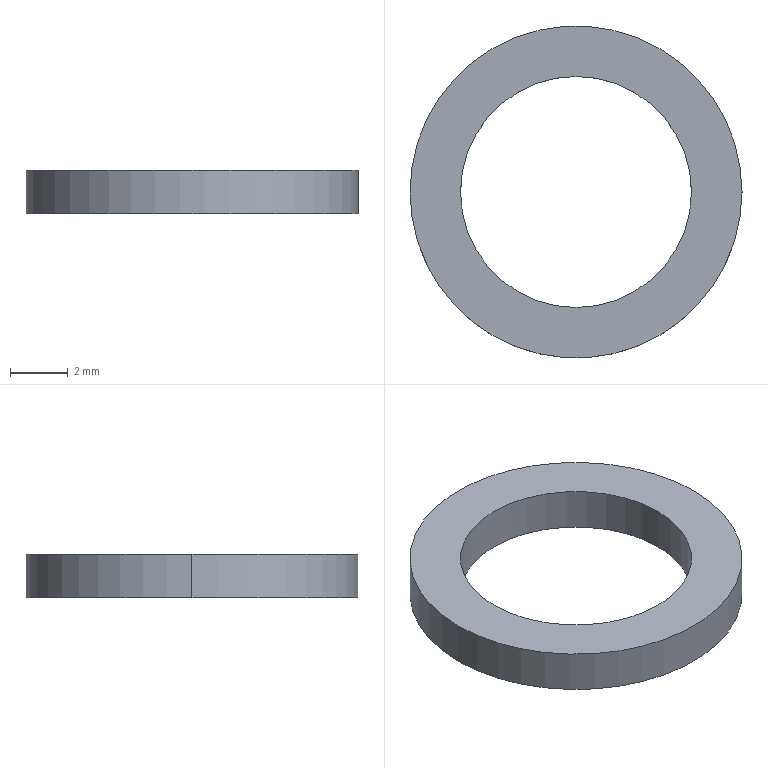Part | NX | features BREP 1 | 1 solid | 6 faces | box 11.5 x 11.5 x 1.5 mm | volume 80.405 mm3 | cylinder 4 | plane 2 | commonest cylinder face diameters 8 x2 11.5 x2
STEP:
#1=CARTESIAN_POINT('',(4.,0.,1.5));
#2=VERTEX_POINT('',#1);
#3=CARTESIAN_POINT('',(4.,0.,0.));
#4=VERTEX_POINT('',#3);
#5=CARTESIAN_POINT('',(4.,0.,1.5));
#6=DIRECTION('',(0.,0.,-1.));
#7=VECTOR('',#6,1000.);
#8=LINE('',#5,#7);
#9=EDGE_CURVE('',#2,#4,#8,.T.);
#10=ORIENTED_EDGE('',*,*,#9,.F.);
#11=CARTESIAN_POINT('',(-4.,0.,1.5));
#12=VERTEX_POINT('',#11);
#13=CARTESIAN_POINT('',(0.,0.,1.5));
#14=DIRECTION('',(0.,0.,1.));
#15=DIRECTION('',(1.,0.,0.));
#16=AXIS2_PLACEMENT_3D('',#13,#14,#15);
#17=CIRCLE('',#16,4.);
#18=EDGE_CURVE('',#2,#12,#17,.T.);
#19=ORIENTED_EDGE('',*,*,#18,.T.);
#20=CARTESIAN_POINT('',(-4.,0.,0.));
#21=VERTEX_POINT('',#20);
#22=CARTESIAN_POINT('',(-4.,0.,1.5));
#23=DIRECTION('',(0.,0.,-1.));
#24=VECTOR('',#23,1000.);
#25=LINE('',#22,#24);
#26=EDGE_CURVE('',#12,#21,#25,.T.);
#27=ORIENTED_EDGE('',*,*,#26,.T.);
#28=CARTESIAN_POINT('',(0.,0.,0.));
#29=DIRECTION('',(0.,0.,1.));
#30=DIRECTION('',(1.,0.,0.));
#31=AXIS2_PLACEMENT_3D('',#28,#29,#30);
#32=CIRCLE('',#31,4.);
#33=EDGE_CURVE('',#4,#21,#32,.T.);
#34=ORIENTED_EDGE('',*,*,#33,.F.);
#35=EDGE_LOOP('',(#10,#19,#27,#34));
#36=FACE_BOUND('',#35,.T.);
#37=CARTESIAN_POINT('',(0.,0.,1.5));
#38=DIRECTION('',(0.,0.,-1.));
#39=DIRECTION('',(-1.,0.,0.));
#40=AXIS2_PLACEMENT_3D('',#37,#38,#39);
#41=CYLINDRICAL_SURFACE('',#40,4.);
#42=ADVANCED_FACE('',(#36),#41,.F.);
#43=CARTESIAN_POINT('',(5.75,0.,1.5));
#44=VERTEX_POINT('',#43);
#45=CARTESIAN_POINT('',(5.75,0.,0.));
#46=VERTEX_POINT('',#45);
#47=CARTESIAN_POINT('',(5.75,0.,1.5));
#48=DIRECTION('',(0.,0.,-1.));
#49=VECTOR('',#48,1000.);
#50=LINE('',#47,#49);
#51=EDGE_CURVE('',#44,#46,#50,.T.);
#52=ORIENTED_EDGE('',*,*,#51,.F.);
#53=CARTESIAN_POINT('',(-5.75,0.,1.5));
#54=VERTEX_POINT('',#53);
#55=CARTESIAN_POINT('',(0.,0.,1.5));
#56=DIRECTION('',(0.,0.,1.));
#57=DIRECTION('',(1.,0.,0.));
#58=AXIS2_PLACEMENT_3D('',#55,#56,#57);
#59=CIRCLE('',#58,5.75);
#60=EDGE_CURVE('',#54,#44,#59,.T.);
#61=ORIENTED_EDGE('',*,*,#60,.F.);
#62=CARTESIAN_POINT('',(-5.75,0.,0.));
#63=VERTEX_POINT('',#62);
#64=CARTESIAN_POINT('',(-5.75,0.,1.5));
#65=DIRECTION('',(0.,0.,-1.));
#66=VECTOR('',#65,1000.);
#67=LINE('',#64,#66);
#68=EDGE_CURVE('',#54,#63,#67,.T.);
#69=ORIENTED_EDGE('',*,*,#68,.T.);
#70=CARTESIAN_POINT('',(0.,0.,0.));
#71=DIRECTION('',(0.,0.,1.));
#72=DIRECTION('',(1.,0.,0.));
#73=AXIS2_PLACEMENT_3D('',#70,#71,#72);
#74=CIRCLE('',#73,5.75);
#75=EDGE_CURVE('',#63,#46,#74,.T.);
#76=ORIENTED_EDGE('',*,*,#75,.T.);
#77=EDGE_LOOP('',(#52,#61,#69,#76));
#78=FACE_BOUND('',#77,.T.);
#79=CARTESIAN_POINT('',(0.,0.,1.5));
#80=DIRECTION('',(0.,0.,-1.));
#81=DIRECTION('',(-1.,0.,0.));
#82=AXIS2_PLACEMENT_3D('',#79,#80,#81);
#83=CYLINDRICAL_SURFACE('',#82,5.75);
#84=ADVANCED_FACE('',(#78),#83,.T.);
#85=CARTESIAN_POINT('',(0.,0.,0.));
#86=DIRECTION('',(0.,0.,1.));
#87=DIRECTION('',(1.,0.,0.));
#88=AXIS2_PLACEMENT_3D('',#85,#86,#87);
#89=CIRCLE('',#88,4.);
#90=EDGE_CURVE('',#21,#4,#89,.T.);
#91=ORIENTED_EDGE('',*,*,#90,.T.);
#92=ORIENTED_EDGE('',*,*,#33,.T.);
#93=EDGE_LOOP('',(#91,#92));
#94=FACE_BOUND('',#93,.T.);
#95=ORIENTED_EDGE('',*,*,#75,.F.);
#96=CARTESIAN_POINT('',(0.,0.,0.));
#97=DIRECTION('',(0.,0.,1.));
#98=DIRECTION('',(1.,0.,0.));
#99=AXIS2_PLACEMENT_3D('',#96,#97,#98);
#100=CIRCLE('',#99,5.75);
#101=EDGE_CURVE('',#46,#63,#100,.T.);
#102=ORIENTED_EDGE('',*,*,#101,.F.);
#103=EDGE_LOOP('',(#95,#102));
#104=FACE_BOUND('',#103,.T.);
#105=CARTESIAN_POINT('',(0.,0.,0.));
#106=DIRECTION('',(0.,0.,1.));
#107=DIRECTION('',(1.,0.,0.));
#108=AXIS2_PLACEMENT_3D('',#105,#106,#107);
#109=PLANE('',#108);
#110=ADVANCED_FACE('',(#94,#104),#109,.F.);
#111=CARTESIAN_POINT('',(0.,0.,1.5));
#112=DIRECTION('',(0.,0.,1.));
#113=DIRECTION('',(1.,0.,0.));
#114=AXIS2_PLACEMENT_3D('',#111,#112,#113);
#115=CIRCLE('',#114,4.);
#116=EDGE_CURVE('',#12,#2,#115,.T.);
#117=ORIENTED_EDGE('',*,*,#116,.F.);
#118=ORIENTED_EDGE('',*,*,#18,.F.);
#119=EDGE_LOOP('',(#117,#118));
#120=FACE_BOUND('',#119,.T.);
#121=ORIENTED_EDGE('',*,*,#60,.T.);
#122=CARTESIAN_POINT('',(0.,0.,1.5));
#123=DIRECTION('',(0.,0.,1.));
#124=DIRECTION('',(1.,0.,0.));
#125=AXIS2_PLACEMENT_3D('',#122,#123,#124);
#126=CIRCLE('',#125,5.75);
#127=EDGE_CURVE('',#44,#54,#126,.T.);
#128=ORIENTED_EDGE('',*,*,#127,.T.);
#129=EDGE_LOOP('',(#121,#128));
#130=FACE_BOUND('',#129,.T.);
#131=CARTESIAN_POINT('',(0.,0.,1.5));
#132=DIRECTION('',(0.,0.,1.));
#133=DIRECTION('',(1.,0.,0.));
#134=AXIS2_PLACEMENT_3D('',#131,#132,#133);
#135=PLANE('',#134);
#136=ADVANCED_FACE('',(#120,#130),#135,.T.);
#137=ORIENTED_EDGE('',*,*,#127,.F.);
#138=ORIENTED_EDGE('',*,*,#51,.T.);
#139=ORIENTED_EDGE('',*,*,#101,.T.);
#140=ORIENTED_EDGE('',*,*,#68,.F.);
#141=EDGE_LOOP('',(#137,#138,#139,#140));
#142=FACE_BOUND('',#141,.T.);
#143=CARTESIAN_POINT('',(0.,0.,1.5));
#144=DIRECTION('',(0.,0.,-1.));
#145=DIRECTION('',(-1.,0.,0.));
#146=AXIS2_PLACEMENT_3D('',#143,#144,#145);
#147=CYLINDRICAL_SURFACE('',#146,5.75);
#148=ADVANCED_FACE('',(#142),#147,.T.);
#149=ORIENTED_EDGE('',*,*,#116,.T.);
#150=ORIENTED_EDGE('',*,*,#9,.T.);
#151=ORIENTED_EDGE('',*,*,#90,.F.);
#152=ORIENTED_EDGE('',*,*,#26,.F.);
#153=EDGE_LOOP('',(#149,#150,#151,#152));
#154=FACE_BOUND('',#153,.T.);
#155=CARTESIAN_POINT('',(0.,0.,1.5));
#156=DIRECTION('',(0.,0.,-1.));
#157=DIRECTION('',(-1.,0.,0.));
#158=AXIS2_PLACEMENT_3D('',#155,#156,#157);
#159=CYLINDRICAL_SURFACE('',#158,4.);
#160=ADVANCED_FACE('',(#154),#159,.F.);
#161=CLOSED_SHELL('',(#42,#84,#110,#136,#148,#160));
#162=MANIFOLD_SOLID_BREP('',#161);
#163=(LENGTH_UNIT()NAMED_UNIT(*)SI_UNIT(.MILLI.,.METRE.));
#164=UNCERTAINTY_MEASURE_WITH_UNIT(LENGTH_MEASURE(0.00001),#163,'','');
#165=(NAMED_UNIT(*)PLANE_ANGLE_UNIT()SI_UNIT($,.RADIAN.));
#166=(NAMED_UNIT(*)SI_UNIT($,.STERADIAN.)SOLID_ANGLE_UNIT());
#167=(GEOMETRIC_REPRESENTATION_CONTEXT(3)GLOBAL_UNCERTAINTY_ASSIGNED_CONTEXT((#164))GLOBAL_UNIT_ASSIGNED_CONTEXT((#163,#165,#166))REPRESENTATION_CONTEXT('',''));
#168=ADVANCED_BREP_SHAPE_REPRESENTATION('',(#162),#167);